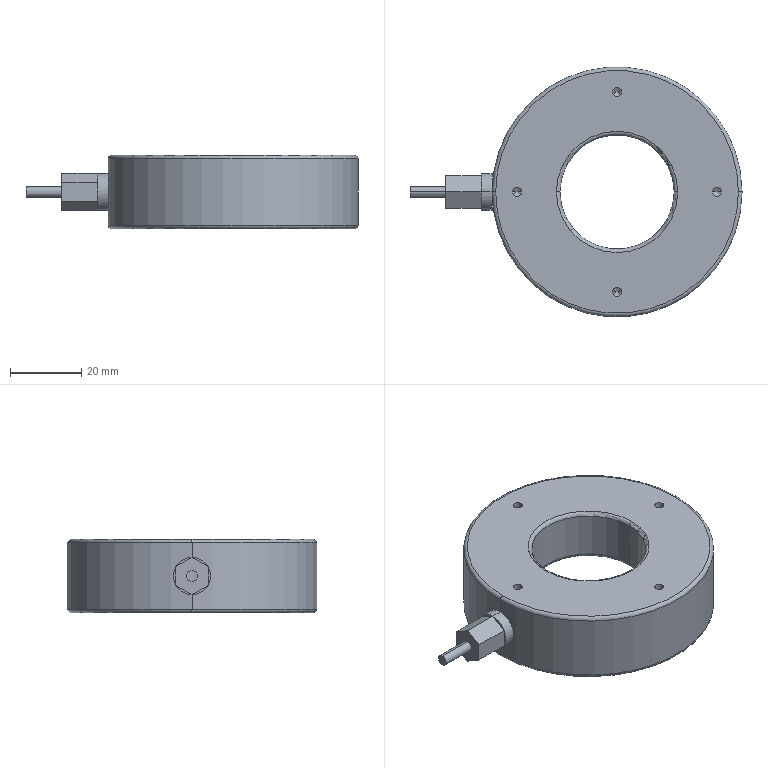Part | STEP file | V-light-HX-A15-D70R3-B-24V | 2 solids | 53 faces | box 93 x 70 x 20.5 mm | volume 59555 mm3 | plane 17 | cylinder 16 | torus 10 | cone 10 | commonest cylinder face diameters 2.5 x8 3 x2 10.4 x2 32 x2 70 x2
STEP:
#1=CARTESIAN_POINT('',(-35.,0.,19.5));
#2=VERTEX_POINT('',#1);
#3=CARTESIAN_POINT('',(35.,0.,19.5));
#4=VERTEX_POINT('',#3);
#5=CARTESIAN_POINT('',(0.,0.,19.5));
#6=DIRECTION('',(0.,0.,-1.));
#7=DIRECTION('',(1.,0.,0.));
#8=AXIS2_PLACEMENT_3D('',#5,#6,#7);
#9=CIRCLE('',#8,35.);
#10=EDGE_CURVE('',#2,#4,#9,.T.);
#11=ORIENTED_EDGE('',*,*,#10,.F.);
#12=CARTESIAN_POINT('',(-34.,0.,20.5));
#13=VERTEX_POINT('',#12);
#14=CARTESIAN_POINT('',(-34.,0.,19.5));
#15=DIRECTION('',(0.,1.,0.));
#16=DIRECTION('',(-1.,0.,0.));
#17=AXIS2_PLACEMENT_3D('',#14,#15,#16);
#18=CIRCLE('',#17,1.);
#19=EDGE_CURVE('',#2,#13,#18,.T.);
#20=ORIENTED_EDGE('',*,*,#19,.T.);
#21=CARTESIAN_POINT('',(34.,0.,20.5));
#22=VERTEX_POINT('',#21);
#23=CARTESIAN_POINT('',(0.,0.,20.5));
#24=DIRECTION('',(0.,0.,1.));
#25=DIRECTION('',(1.,0.,0.));
#26=AXIS2_PLACEMENT_3D('',#23,#24,#25);
#27=CIRCLE('',#26,34.);
#28=EDGE_CURVE('',#22,#13,#27,.T.);
#29=ORIENTED_EDGE('',*,*,#28,.F.);
#30=CARTESIAN_POINT('',(34.,0.,19.5));
#31=DIRECTION('',(0.,-1.,0.));
#32=DIRECTION('',(0.,0.,-1.));
#33=AXIS2_PLACEMENT_3D('',#30,#31,#32);
#34=CIRCLE('',#33,1.);
#35=EDGE_CURVE('',#4,#22,#34,.T.);
#36=ORIENTED_EDGE('',*,*,#35,.F.);
#37=EDGE_LOOP('',(#11,#20,#29,#36));
#38=FACE_OUTER_BOUND('',#37,.T.);
#39=CARTESIAN_POINT('',(0.,0.,19.5));
#40=DIRECTION('',(0.,0.,1.));
#41=DIRECTION('',(1.,0.,0.));
#42=AXIS2_PLACEMENT_3D('',#39,#40,#41);
#43=TOROIDAL_SURFACE('',#42,34.,1.);
#44=ADVANCED_FACE('',(#38),#43,.T.);
#45=CARTESIAN_POINT('',(-34.,0.,0.));
#46=VERTEX_POINT('',#45);
#47=CARTESIAN_POINT('',(34.,0.,0.));
#48=VERTEX_POINT('',#47);
#49=CARTESIAN_POINT('',(0.,0.,0.));
#50=DIRECTION('',(0.,0.,-1.));
#51=DIRECTION('',(1.,0.,0.));
#52=AXIS2_PLACEMENT_3D('',#49,#50,#51);
#53=CIRCLE('',#52,34.);
#54=EDGE_CURVE('',#46,#48,#53,.T.);
#55=ORIENTED_EDGE('',*,*,#54,.F.);
#56=CARTESIAN_POINT('',(-35.,0.,1.));
#57=VERTEX_POINT('',#56);
#58=CARTESIAN_POINT('',(-34.,0.,1.));
#59=DIRECTION('',(0.,1.,0.));
#60=DIRECTION('',(-1.,0.,0.));
#61=AXIS2_PLACEMENT_3D('',#58,#59,#60);
#62=CIRCLE('',#61,1.);
#63=EDGE_CURVE('',#46,#57,#62,.T.);
#64=ORIENTED_EDGE('',*,*,#63,.T.);
#65=CARTESIAN_POINT('',(35.,0.,1.));
#66=VERTEX_POINT('',#65);
#67=CARTESIAN_POINT('',(0.,0.,1.));
#68=DIRECTION('',(0.,0.,1.));
#69=DIRECTION('',(1.,0.,0.));
#70=AXIS2_PLACEMENT_3D('',#67,#68,#69);
#71=CIRCLE('',#70,35.);
#72=EDGE_CURVE('',#66,#57,#71,.T.);
#73=ORIENTED_EDGE('',*,*,#72,.F.);
#74=CARTESIAN_POINT('',(34.,0.,1.));
#75=DIRECTION('',(0.,-1.,0.));
#76=DIRECTION('',(0.,0.,-1.));
#77=AXIS2_PLACEMENT_3D('',#74,#75,#76);
#78=CIRCLE('',#77,1.);
#79=EDGE_CURVE('',#48,#66,#78,.T.);
#80=ORIENTED_EDGE('',*,*,#79,.F.);
#81=EDGE_LOOP('',(#55,#64,#73,#80));
#82=FACE_OUTER_BOUND('',#81,.T.);
#83=CARTESIAN_POINT('',(0.,0.,1.));
#84=DIRECTION('',(0.,0.,1.));
#85=DIRECTION('',(1.,0.,0.));
#86=AXIS2_PLACEMENT_3D('',#83,#84,#85);
#87=TOROIDAL_SURFACE('',#86,34.,1.);
#88=ADVANCED_FACE('',(#82),#87,.T.);
#89=CARTESIAN_POINT('',(-16.,0.,6.566));
#90=VERTEX_POINT('',#89);
#91=CARTESIAN_POINT('',(16.,0.,6.566));
#92=VERTEX_POINT('',#91);
#93=CARTESIAN_POINT('',(0.,0.,6.566));
#94=DIRECTION('',(0.,0.,-1.));
#95=DIRECTION('',(1.,0.,0.));
#96=AXIS2_PLACEMENT_3D('',#93,#94,#95);
#97=CIRCLE('',#96,16.);
#98=EDGE_CURVE('',#90,#92,#97,.T.);
#99=ORIENTED_EDGE('',*,*,#98,.F.);
#100=CARTESIAN_POINT('',(-16.486,0.,5.709));
#101=VERTEX_POINT('',#100);
#102=CARTESIAN_POINT('',(-17.,0.,6.566));
#103=DIRECTION('',(0.,1.,0.));
#104=DIRECTION('',(-1.,0.,0.));
#105=AXIS2_PLACEMENT_3D('',#102,#103,#104);
#106=CIRCLE('',#105,1.);
#107=EDGE_CURVE('',#90,#101,#106,.T.);
#108=ORIENTED_EDGE('',*,*,#107,.T.);
#109=CARTESIAN_POINT('',(16.486,0.,5.709));
#110=VERTEX_POINT('',#109);
#111=CARTESIAN_POINT('',(0.,0.,5.709));
#112=DIRECTION('',(0.,0.,1.));
#113=DIRECTION('',(1.,0.,0.));
#114=AXIS2_PLACEMENT_3D('',#111,#112,#113);
#115=CIRCLE('',#114,16.486);
#116=EDGE_CURVE('',#110,#101,#115,.T.);
#117=ORIENTED_EDGE('',*,*,#116,.F.);
#118=CARTESIAN_POINT('',(17.,0.,6.566));
#119=DIRECTION('',(0.,-1.,0.));
#120=DIRECTION('',(0.,0.,-1.));
#121=AXIS2_PLACEMENT_3D('',#118,#119,#120);
#122=CIRCLE('',#121,1.);
#123=EDGE_CURVE('',#92,#110,#122,.T.);
#124=ORIENTED_EDGE('',*,*,#123,.F.);
#125=EDGE_LOOP('',(#99,#108,#117,#124));
#126=FACE_OUTER_BOUND('',#125,.T.);
#127=CARTESIAN_POINT('',(0.,0.,6.566));
#128=DIRECTION('',(0.,0.,1.));
#129=DIRECTION('',(1.,0.,0.));
#130=AXIS2_PLACEMENT_3D('',#127,#128,#129);
#131=TOROIDAL_SURFACE('',#130,17.,1.);
#132=ADVANCED_FACE('',(#126),#131,.T.);
#133=CARTESIAN_POINT('',(-17.,0.,20.5));
#134=VERTEX_POINT('',#133);
#135=CARTESIAN_POINT('',(17.,0.,20.5));
#136=VERTEX_POINT('',#135);
#137=CARTESIAN_POINT('',(0.,0.,20.5));
#138=DIRECTION('',(0.,0.,-1.));
#139=DIRECTION('',(1.,0.,0.));
#140=AXIS2_PLACEMENT_3D('',#137,#138,#139);
#141=CIRCLE('',#140,17.);
#142=EDGE_CURVE('',#134,#136,#141,.T.);
#143=ORIENTED_EDGE('',*,*,#142,.F.);
#144=CARTESIAN_POINT('',(-16.,0.,19.5));
#145=VERTEX_POINT('',#144);
#146=CARTESIAN_POINT('',(-17.,0.,19.5));
#147=DIRECTION('',(0.,1.,0.));
#148=DIRECTION('',(-1.,0.,0.));
#149=AXIS2_PLACEMENT_3D('',#146,#147,#148);
#150=CIRCLE('',#149,1.);
#151=EDGE_CURVE('',#134,#145,#150,.T.);
#152=ORIENTED_EDGE('',*,*,#151,.T.);
#153=CARTESIAN_POINT('',(16.,0.,19.5));
#154=VERTEX_POINT('',#153);
#155=CARTESIAN_POINT('',(0.,0.,19.5));
#156=DIRECTION('',(0.,0.,1.));
#157=DIRECTION('',(1.,0.,0.));
#158=AXIS2_PLACEMENT_3D('',#155,#156,#157);
#159=CIRCLE('',#158,16.);
#160=EDGE_CURVE('',#154,#145,#159,.T.);
#161=ORIENTED_EDGE('',*,*,#160,.F.);
#162=CARTESIAN_POINT('',(17.,0.,19.5));
#163=DIRECTION('',(0.,-1.,0.));
#164=DIRECTION('',(0.,0.,-1.));
#165=AXIS2_PLACEMENT_3D('',#162,#163,#164);
#166=CIRCLE('',#165,1.);
#167=EDGE_CURVE('',#136,#154,#166,.T.);
#168=ORIENTED_EDGE('',*,*,#167,.F.);
#169=EDGE_LOOP('',(#143,#152,#161,#168));
#170=FACE_OUTER_BOUND('',#169,.T.);
#171=CARTESIAN_POINT('',(0.,0.,19.5));
#172=DIRECTION('',(0.,0.,1.));
#173=DIRECTION('',(1.,0.,0.));
#174=AXIS2_PLACEMENT_3D('',#171,#172,#173);
#175=TOROIDAL_SURFACE('',#174,17.,1.);
#176=ADVANCED_FACE('',(#170),#175,.T.);
#177=CARTESIAN_POINT('',(-25.762,0.,0.1425));
#178=VERTEX_POINT('',#177);
#179=CARTESIAN_POINT('',(25.762,0.,0.1425));
#180=VERTEX_POINT('',#179);
#181=CARTESIAN_POINT('',(0.,0.,0.1425));
#182=DIRECTION('',(0.,0.,-1.));
#183=DIRECTION('',(-1.,0.,0.));
#184=AXIS2_PLACEMENT_3D('',#181,#182,#183);
#185=CIRCLE('',#184,25.762);
#186=EDGE_CURVE('',#178,#180,#185,.T.);
#187=ORIENTED_EDGE('',*,*,#186,.F.);
#188=CARTESIAN_POINT('',(-26.277,0.,0.));
#189=VERTEX_POINT('',#188);
#190=CARTESIAN_POINT('',(-26.277,0.,1.));
#191=DIRECTION('',(0.,1.,0.));
#192=DIRECTION('',(-1.,0.,0.));
#193=AXIS2_PLACEMENT_3D('',#190,#191,#192);
#194=CIRCLE('',#193,1.);
#195=EDGE_CURVE('',#178,#189,#194,.T.);
#196=ORIENTED_EDGE('',*,*,#195,.T.);
#197=CARTESIAN_POINT('',(26.277,0.,0.));
#198=VERTEX_POINT('',#197);
#199=CARTESIAN_POINT('',(0.,0.,0.));
#200=DIRECTION('',(0.,0.,1.));
#201=DIRECTION('',(1.,0.,0.));
#202=AXIS2_PLACEMENT_3D('',#199,#200,#201);
#203=CIRCLE('',#202,26.277);
#204=EDGE_CURVE('',#198,#189,#203,.T.);
#205=ORIENTED_EDGE('',*,*,#204,.F.);
#206=CARTESIAN_POINT('',(26.277,0.,1.));
#207=DIRECTION('',(0.,-1.,0.));
#208=DIRECTION('',(0.,0.,-1.));
#209=AXIS2_PLACEMENT_3D('',#206,#207,#208);
#210=CIRCLE('',#209,1.);
#211=EDGE_CURVE('',#180,#198,#210,.T.);
#212=ORIENTED_EDGE('',*,*,#211,.F.);
#213=EDGE_LOOP('',(#187,#196,#205,#212));
#214=FACE_OUTER_BOUND('',#213,.T.);
#215=CARTESIAN_POINT('',(0.,0.,1.));
#216=DIRECTION('',(0.,0.,1.));
#217=DIRECTION('',(1.,0.,0.));
#218=AXIS2_PLACEMENT_3D('',#215,#216,#217);
#219=TOROIDAL_SURFACE('',#218,26.277,1.);
#220=ADVANCED_FACE('',(#214),#219,.T.);
#221=CARTESIAN_POINT('',(0.,0.,5.709));
#222=DIRECTION('',(0.,0.,1.));
#223=DIRECTION('',(1.,0.,0.));
#224=AXIS2_PLACEMENT_3D('',#221,#222,#223);
#225=CIRCLE('',#224,16.486);
#226=EDGE_CURVE('',#101,#110,#225,.T.);
#227=ORIENTED_EDGE('',*,*,#226,.T.);
#228=CARTESIAN_POINT('',(26.,0.,0.));
#229=DIRECTION('',(0.8575,0.,-0.5145));
#230=VECTOR('',#229,1000.);
#231=LINE('',#228,#230);
#232=EDGE_CURVE('',#110,#180,#231,.T.);
#233=ORIENTED_EDGE('',*,*,#232,.T.);
#234=CARTESIAN_POINT('',(0.,0.,0.1425));
#235=DIRECTION('',(0.,0.,-1.));
#236=DIRECTION('',(-1.,0.,0.));
#237=AXIS2_PLACEMENT_3D('',#234,#235,#236);
#238=CIRCLE('',#237,25.762);
#239=EDGE_CURVE('',#180,#178,#238,.T.);
#240=ORIENTED_EDGE('',*,*,#239,.T.);
#241=CARTESIAN_POINT('',(-26.,0.,0.));
#242=DIRECTION('',(-0.8575,0.,-0.5145));
#243=VECTOR('',#242,1000.);
#244=LINE('',#241,#243);
#245=EDGE_CURVE('',#101,#178,#244,.T.);
#246=ORIENTED_EDGE('',*,*,#245,.F.);
#247=EDGE_LOOP('',(#227,#233,#240,#246));
#248=FACE_OUTER_BOUND('',#247,.T.);
#249=CARTESIAN_POINT('',(0.,0.,0.));
#250=DIRECTION('',(0.,0.,-1.));
#251=DIRECTION('',(-1.,0.,0.));
#252=AXIS2_PLACEMENT_3D('',#249,#250,#251);
#253=CONICAL_SURFACE('',#252,26.,1.03);
#254=ADVANCED_FACE('',(#248),#253,.F.);
#255=CARTESIAN_POINT('',(-1.25,28.,15.));
#256=VERTEX_POINT('',#255);
#257=CARTESIAN_POINT('',(1.25,28.,15.));
#258=VERTEX_POINT('',#257);
#259=CARTESIAN_POINT('',(0.,28.,15.));
#260=DIRECTION('',(0.,0.,1.));
#261=DIRECTION('',(1.,0.,0.));
#262=AXIS2_PLACEMENT_3D('',#259,#260,#261);
#263=CIRCLE('',#262,1.25);
#264=EDGE_CURVE('',#256,#258,#263,.T.);
#265=ORIENTED_EDGE('',*,*,#264,.F.);
#266=CARTESIAN_POINT('',(-1.25,28.,20.5));
#267=VERTEX_POINT('',#266);
#268=CARTESIAN_POINT('',(-1.25,28.,20.5));
#269=DIRECTION('',(0.,0.,1.));
#270=VECTOR('',#269,1000.);
#271=LINE('',#268,#270);
#272=EDGE_CURVE('',#256,#267,#271,.T.);
#273=ORIENTED_EDGE('',*,*,#272,.T.);
#274=CARTESIAN_POINT('',(1.25,28.,20.5));
#275=VERTEX_POINT('',#274);
#276=CARTESIAN_POINT('',(0.,28.,20.5));
#277=DIRECTION('',(0.,0.,1.));
#278=DIRECTION('',(1.,0.,0.));
#279=AXIS2_PLACEMENT_3D('',#276,#277,#278);
#280=CIRCLE('',#279,1.25);
#281=EDGE_CURVE('',#267,#275,#280,.T.);
#282=ORIENTED_EDGE('',*,*,#281,.T.);
#283=CARTESIAN_POINT('',(1.25,28.,20.5));
#284=DIRECTION('',(0.,0.,1.));
#285=VECTOR('',#284,1000.);
#286=LINE('',#283,#285);
#287=EDGE_CURVE('',#258,#275,#286,.T.);
#288=ORIENTED_EDGE('',*,*,#287,.F.);
#289=EDGE_LOOP('',(#265,#273,#282,#288));
#290=FACE_OUTER_BOUND('',#289,.T.);
#291=CARTESIAN_POINT('',(0.,28.,20.5));
#292=DIRECTION('',(0.,0.,1.));
#293=DIRECTION('',(1.,0.,0.));
#294=AXIS2_PLACEMENT_3D('',#291,#292,#293);
#295=CYLINDRICAL_SURFACE('',#294,1.25);
#296=ADVANCED_FACE('',(#290),#295,.F.);
#297=CARTESIAN_POINT('',(0.,28.,14.249));
#298=VERTEX_POINT('',#297);
#299=CARTESIAN_POINT('',(1.25,28.,15.));
#300=DIRECTION('',(0.8572,0.,0.515));
#301=VECTOR('',#300,1000.);
#302=LINE('',#299,#301);
#303=EDGE_CURVE('',#298,#258,#302,.T.);
#304=ORIENTED_EDGE('',*,*,#303,.F.);
#305=CARTESIAN_POINT('',(-1.25,28.,15.));
#306=DIRECTION('',(-0.8572,0.,0.515));
#307=VECTOR('',#306,1000.);
#308=LINE('',#305,#307);
#309=EDGE_CURVE('',#298,#256,#308,.T.);
#310=ORIENTED_EDGE('',*,*,#309,.T.);
#311=ORIENTED_EDGE('',*,*,#264,.T.);
#312=EDGE_LOOP('',(#304,#310,#311));
#313=FACE_OUTER_BOUND('',#312,.T.);
#314=CARTESIAN_POINT('',(0.,28.,15.));
#315=DIRECTION('',(0.,0.,1.));
#316=DIRECTION('',(1.,0.,0.));
#317=AXIS2_PLACEMENT_3D('',#314,#315,#316);
#318=CONICAL_SURFACE('',#317,1.25,1.03);
#319=ADVANCED_FACE('',(#313),#318,.F.);
#320=CARTESIAN_POINT('',(26.75,0.,15.));
#321=VERTEX_POINT('',#320);
#322=CARTESIAN_POINT('',(29.25,0.,15.));
#323=VERTEX_POINT('',#322);
#324=CARTESIAN_POINT('',(28.,0.,15.));
#325=DIRECTION('',(0.,0.,1.));
#326=DIRECTION('',(1.,0.,0.));
#327=AXIS2_PLACEMENT_3D('',#324,#325,#326);
#328=CIRCLE('',#327,1.25);
#329=EDGE_CURVE('',#321,#323,#328,.T.);
#330=ORIENTED_EDGE('',*,*,#329,.F.);
#331=CARTESIAN_POINT('',(26.75,0.,20.5));
#332=VERTEX_POINT('',#331);
#333=CARTESIAN_POINT('',(26.75,0.,20.5));
#334=DIRECTION('',(0.,0.,1.));
#335=VECTOR('',#334,1000.);
#336=LINE('',#333,#335);
#337=EDGE_CURVE('',#321,#332,#336,.T.);
#338=ORIENTED_EDGE('',*,*,#337,.T.);
#339=CARTESIAN_POINT('',(29.25,0.,20.5));
#340=VERTEX_POINT('',#339);
#341=CARTESIAN_POINT('',(28.,0.,20.5));
#342=DIRECTION('',(0.,0.,1.));
#343=DIRECTION('',(1.,0.,0.));
#344=AXIS2_PLACEMENT_3D('',#341,#342,#343);
#345=CIRCLE('',#344,1.25);
#346=EDGE_CURVE('',#332,#340,#345,.T.);
#347=ORIENTED_EDGE('',*,*,#346,.T.);
#348=CARTESIAN_POINT('',(29.25,0.,20.5));
#349=DIRECTION('',(0.,0.,1.));
#350=VECTOR('',#349,1000.);
#351=LINE('',#348,#350);
#352=EDGE_CURVE('',#323,#340,#351,.T.);
#353=ORIENTED_EDGE('',*,*,#352,.F.);
#354=EDGE_LOOP('',(#330,#338,#347,#353));
#355=FACE_OUTER_BOUND('',#354,.T.);
#356=CARTESIAN_POINT('',(28.,0.,20.5));
#357=DIRECTION('',(0.,0.,1.));
#358=DIRECTION('',(1.,0.,0.));
#359=AXIS2_PLACEMENT_3D('',#356,#357,#358);
#360=CYLINDRICAL_SURFACE('',#359,1.25);
#361=ADVANCED_FACE('',(#355),#360,.F.);
#362=CARTESIAN_POINT('',(28.,0.,14.249));
#363=VERTEX_POINT('',#362);
#364=CARTESIAN_POINT('',(29.25,0.,15.));
#365=DIRECTION('',(0.8572,0.,0.515));
#366=VECTOR('',#365,1000.);
#367=LINE('',#364,#366);
#368=EDGE_CURVE('',#363,#323,#367,.T.);
#369=ORIENTED_EDGE('',*,*,#368,.F.);
#370=CARTESIAN_POINT('',(26.75,0.,15.));
#371=DIRECTION('',(-0.8572,0.,0.515));
#372=VECTOR('',#371,1000.);
#373=LINE('',#370,#372);
#374=EDGE_CURVE('',#363,#321,#373,.T.);
#375=ORIENTED_EDGE('',*,*,#374,.T.);
#376=ORIENTED_EDGE('',*,*,#329,.T.);
#377=EDGE_LOOP('',(#369,#375,#376));
#378=FACE_OUTER_BOUND('',#377,.T.);
#379=CARTESIAN_POINT('',(28.,0.,15.));
#380=DIRECTION('',(0.,0.,1.));
#381=DIRECTION('',(1.,0.,0.));
#382=AXIS2_PLACEMENT_3D('',#379,#380,#381);
#383=CONICAL_SURFACE('',#382,1.25,1.03);
#384=ADVANCED_FACE('',(#378),#383,.F.);
#385=CARTESIAN_POINT('',(-1.25,-28.,15.));
#386=VERTEX_POINT('',#385);
#387=CARTESIAN_POINT('',(1.25,-28.,15.));
#388=VERTEX_POINT('',#387);
#389=CARTESIAN_POINT('',(0.,-28.,15.));
#390=DIRECTION('',(0.,0.,1.));
#391=DIRECTION('',(1.,0.,0.));
#392=AXIS2_PLACEMENT_3D('',#389,#390,#391);
#393=CIRCLE('',#392,1.25);
#394=EDGE_CURVE('',#386,#388,#393,.T.);
#395=ORIENTED_EDGE('',*,*,#394,.F.);
#396=CARTESIAN_POINT('',(-1.25,-28.,20.5));
#397=VERTEX_POINT('',#396);
#398=CARTESIAN_POINT('',(-1.25,-28.,20.5));
#399=DIRECTION('',(0.,0.,1.));
#400=VECTOR('',#399,1000.);
#401=LINE('',#398,#400);
#402=EDGE_CURVE('',#386,#397,#401,.T.);
#403=ORIENTED_EDGE('',*,*,#402,.T.);
#404=CARTESIAN_POINT('',(1.25,-28.,20.5));
#405=VERTEX_POINT('',#404);
#406=CARTESIAN_POINT('',(0.,-28.,20.5));
#407=DIRECTION('',(0.,0.,1.));
#408=DIRECTION('',(1.,0.,0.));
#409=AXIS2_PLACEMENT_3D('',#406,#407,#408);
#410=CIRCLE('',#409,1.25);
#411=EDGE_CURVE('',#397,#405,#410,.T.);
#412=ORIENTED_EDGE('',*,*,#411,.T.);
#413=CARTESIAN_POINT('',(1.25,-28.,20.5));
#414=DIRECTION('',(0.,0.,1.));
#415=VECTOR('',#414,1000.);
#416=LINE('',#413,#415);
#417=EDGE_CURVE('',#388,#405,#416,.T.);
#418=ORIENTED_EDGE('',*,*,#417,.F.);
#419=EDGE_LOOP('',(#395,#403,#412,#418));
#420=FACE_OUTER_BOUND('',#419,.T.);
#421=CARTESIAN_POINT('',(0.,-28.,20.5));
#422=DIRECTION('',(0.,0.,1.));
#423=DIRECTION('',(1.,0.,0.));
#424=AXIS2_PLACEMENT_3D('',#421,#422,#423);
#425=CYLINDRICAL_SURFACE('',#424,1.25);
#426=ADVANCED_FACE('',(#420),#425,.F.);
#427=CARTESIAN_POINT('',(0.,-28.,14.249));
#428=VERTEX_POINT('',#427);
#429=CARTESIAN_POINT('',(1.25,-28.,15.));
#430=DIRECTION('',(0.8572,0.,0.515));
#431=VECTOR('',#430,1000.);
#432=LINE('',#429,#431);
#433=EDGE_CURVE('',#428,#388,#432,.T.);
#434=ORIENTED_EDGE('',*,*,#433,.F.);
#435=CARTESIAN_POINT('',(-1.25,-28.,15.));
#436=DIRECTION('',(-0.8572,0.,0.515));
#437=VECTOR('',#436,1000.);
#438=LINE('',#435,#437);
#439=EDGE_CURVE('',#428,#386,#438,.T.);
#440=ORIENTED_EDGE('',*,*,#439,.T.);
#441=ORIENTED_EDGE('',*,*,#394,.T.);
#442=EDGE_LOOP('',(#434,#440,#441));
#443=FACE_OUTER_BOUND('',#442,.T.);
#444=CARTESIAN_POINT('',(0.,-28.,15.));
#445=DIRECTION('',(0.,0.,1.));
#446=DIRECTION('',(1.,0.,0.));
#447=AXIS2_PLACEMENT_3D('',#444,#445,#446);
#448=CONICAL_SURFACE('',#447,1.25,1.03);
#449=ADVANCED_FACE('',(#443),#448,.F.);
#450=CARTESIAN_POINT('',(-29.25,0.,15.));
#451=VERTEX_POINT('',#450);
#452=CARTESIAN_POINT('',(-26.75,0.,15.));
#453=VERTEX_POINT('',#452);
#454=CARTESIAN_POINT('',(-28.,0.,15.));
#455=DIRECTION('',(0.,0.,1.));
#456=DIRECTION('',(1.,0.,0.));
#457=AXIS2_PLACEMENT_3D('',#454,#455,#456);
#458=CIRCLE('',#457,1.25);
#459=EDGE_CURVE('',#451,#453,#458,.T.);
#460=ORIENTED_EDGE('',*,*,#459,.F.);
#461=CARTESIAN_POINT('',(-29.25,0.,20.5));
#462=VERTEX_POINT('',#461);
#463=CARTESIAN_POINT('',(-29.25,0.,20.5));
#464=DIRECTION('',(0.,0.,1.));
#465=VECTOR('',#464,1000.);
#466=LINE('',#463,#465);
#467=EDGE_CURVE('',#451,#462,#466,.T.);
#468=ORIENTED_EDGE('',*,*,#467,.T.);
#469=CARTESIAN_POINT('',(-26.75,0.,20.5));
#470=VERTEX_POINT('',#469);
#471=CARTESIAN_POINT('',(-28.,0.,20.5));
#472=DIRECTION('',(0.,0.,1.));
#473=DIRECTION('',(1.,0.,0.));
#474=AXIS2_PLACEMENT_3D('',#471,#472,#473);
#475=CIRCLE('',#474,1.25);
#476=EDGE_CURVE('',#462,#470,#475,.T.);
#477=ORIENTED_EDGE('',*,*,#476,.T.);
#478=CARTESIAN_POINT('',(-26.75,0.,20.5));
#479=DIRECTION('',(0.,0.,1.));
#480=VECTOR('',#479,1000.);
#481=LINE('',#478,#480);
#482=EDGE_CURVE('',#453,#470,#481,.T.);
#483=ORIENTED_EDGE('',*,*,#482,.F.);
#484=EDGE_LOOP('',(#460,#468,#477,#483));
#485=FACE_OUTER_BOUND('',#484,.T.);
#486=CARTESIAN_POINT('',(-28.,0.,20.5));
#487=DIRECTION('',(0.,0.,1.));
#488=DIRECTION('',(1.,0.,0.));
#489=AXIS2_PLACEMENT_3D('',#486,#487,#488);
#490=CYLINDRICAL_SURFACE('',#489,1.25);
#491=ADVANCED_FACE('',(#485),#490,.F.);
#492=CARTESIAN_POINT('',(-28.,0.,14.249));
#493=VERTEX_POINT('',#492);
#494=CARTESIAN_POINT('',(-26.75,0.,15.));
#495=DIRECTION('',(0.8572,0.,0.515));
#496=VECTOR('',#495,1000.);
#497=LINE('',#494,#496);
#498=EDGE_CURVE('',#493,#453,#497,.T.);
#499=ORIENTED_EDGE('',*,*,#498,.F.);
#500=CARTESIAN_POINT('',(-29.25,0.,15.));
#501=DIRECTION('',(-0.8572,0.,0.515));
#502=VECTOR('',#501,1000.);
#503=LINE('',#500,#502);
#504=EDGE_CURVE('',#493,#451,#503,.T.);
#505=ORIENTED_EDGE('',*,*,#504,.T.);
#506=ORIENTED_EDGE('',*,*,#459,.T.);
#507=EDGE_LOOP('',(#499,#505,#506));
#508=FACE_OUTER_BOUND('',#507,.T.);
#509=CARTESIAN_POINT('',(-28.,0.,15.));
#510=DIRECTION('',(0.,0.,1.));
#511=DIRECTION('',(1.,0.,0.));
#512=AXIS2_PLACEMENT_3D('',#509,#510,#511);
#513=CONICAL_SURFACE('',#512,1.25,1.03);
#514=ADVANCED_FACE('',(#508),#513,.F.);
#515=CARTESIAN_POINT('',(0.,0.,19.5));
#516=DIRECTION('',(0.,0.,1.));
#517=DIRECTION('',(1.,0.,0.));
#518=AXIS2_PLACEMENT_3D('',#515,#516,#517);
#519=CIRCLE('',#518,16.);
#520=EDGE_CURVE('',#145,#154,#519,.T.);
#521=ORIENTED_EDGE('',*,*,#520,.T.);
#522=CARTESIAN_POINT('',(16.,0.,20.5));
#523=DIRECTION('',(0.,0.,-1.));
#524=VECTOR('',#523,1000.);
#525=LINE('',#522,#524);
#526=EDGE_CURVE('',#154,#92,#525,.T.);
#527=ORIENTED_EDGE('',*,*,#526,.T.);
#528=CARTESIAN_POINT('',(0.,0.,6.566));
#529=DIRECTION('',(0.,0.,-1.));
#530=DIRECTION('',(1.,0.,0.));
#531=AXIS2_PLACEMENT_3D('',#528,#529,#530);
#532=CIRCLE('',#531,16.);
#533=EDGE_CURVE('',#92,#90,#532,.T.);
#534=ORIENTED_EDGE('',*,*,#533,.T.);
#535=CARTESIAN_POINT('',(-16.,0.,20.5));
#536=DIRECTION('',(0.,0.,-1.));
#537=VECTOR('',#536,1000.);
#538=LINE('',#535,#537);
#539=EDGE_CURVE('',#145,#90,#538,.T.);
#540=ORIENTED_EDGE('',*,*,#539,.F.);
#541=EDGE_LOOP('',(#521,#527,#534,#540));
#542=FACE_OUTER_BOUND('',#541,.T.);
#543=CARTESIAN_POINT('',(0.,0.,20.5));
#544=DIRECTION('',(0.,0.,-1.));
#545=DIRECTION('',(-1.,0.,0.));
#546=AXIS2_PLACEMENT_3D('',#543,#544,#545);
#547=CYLINDRICAL_SURFACE('',#546,16.);
#548=ADVANCED_FACE('',(#542),#547,.F.);
#549=ORIENTED_EDGE('',*,*,#10,.T.);
#550=CARTESIAN_POINT('',(35.,0.,20.5));
#551=DIRECTION('',(0.,0.,-1.));
#552=VECTOR('',#551,1000.);
#553=LINE('',#550,#552);
#554=EDGE_CURVE('',#4,#66,#553,.T.);
#555=ORIENTED_EDGE('',*,*,#554,.T.);
#556=ORIENTED_EDGE('',*,*,#72,.T.);
#557=CARTESIAN_POINT('',(-35.,0.,20.5));
#558=DIRECTION('',(0.,0.,-1.));
#559=VECTOR('',#558,1000.);
#560=LINE('',#557,#559);
#561=EDGE_CURVE('',#2,#57,#560,.T.);
#562=ORIENTED_EDGE('',*,*,#561,.F.);
#563=EDGE_LOOP('',(#549,#555,#556,#562));
#564=FACE_OUTER_BOUND('',#563,.T.);
#565=CARTESIAN_POINT('',(0.,0.,20.5));
#566=DIRECTION('',(0.,0.,-1.));
#567=DIRECTION('',(-1.,0.,0.));
#568=AXIS2_PLACEMENT_3D('',#565,#566,#567);
#569=CYLINDRICAL_SURFACE('',#568,35.);
#570=ADVANCED_FACE('',(#564),#569,.T.);
#571=CARTESIAN_POINT('',(0.,0.,20.5));
#572=DIRECTION('',(0.,0.,-1.));
#573=DIRECTION('',(1.,0.,0.));
#574=AXIS2_PLACEMENT_3D('',#571,#572,#573);
#575=CIRCLE('',#574,17.);
#576=EDGE_CURVE('',#136,#134,#575,.T.);
#577=ORIENTED_EDGE('',*,*,#576,.T.);
#578=ORIENTED_EDGE('',*,*,#142,.T.);
#579=EDGE_LOOP('',(#577,#578));
#580=FACE_BOUND('',#579,.T.);
#581=ORIENTED_EDGE('',*,*,#28,.T.);
#582=CARTESIAN_POINT('',(0.,0.,20.5));
#583=DIRECTION('',(0.,0.,1.));
#584=DIRECTION('',(1.,0.,0.));
#585=AXIS2_PLACEMENT_3D('',#582,#583,#584);
#586=CIRCLE('',#585,34.);
#587=EDGE_CURVE('',#13,#22,#586,.T.);
#588=ORIENTED_EDGE('',*,*,#587,.T.);
#589=EDGE_LOOP('',(#581,#588));
#590=FACE_OUTER_BOUND('',#589,.T.);
#591=CARTESIAN_POINT('',(0.,28.,20.5));
#592=DIRECTION('',(0.,0.,1.));
#593=DIRECTION('',(1.,0.,0.));
#594=AXIS2_PLACEMENT_3D('',#591,#592,#593);
#595=CIRCLE('',#594,1.25);
#596=EDGE_CURVE('',#275,#267,#595,.T.);
#597=ORIENTED_EDGE('',*,*,#596,.F.);
#598=ORIENTED_EDGE('',*,*,#281,.F.);
#599=EDGE_LOOP('',(#597,#598));
#600=FACE_BOUND('',#599,.T.);
#601=CARTESIAN_POINT('',(28.,0.,20.5));
#602=DIRECTION('',(0.,0.,1.));
#603=DIRECTION('',(1.,0.,0.));
#604=AXIS2_PLACEMENT_3D('',#601,#602,#603);
#605=CIRCLE('',#604,1.25);
#606=EDGE_CURVE('',#340,#332,#605,.T.);
#607=ORIENTED_EDGE('',*,*,#606,.F.);
#608=ORIENTED_EDGE('',*,*,#346,.F.);
#609=EDGE_LOOP('',(#607,#608));
#610=FACE_BOUND('',#609,.T.);
#611=CARTESIAN_POINT('',(0.,-28.,20.5));
#612=DIRECTION('',(0.,0.,1.));
#613=DIRECTION('',(1.,0.,0.));
#614=AXIS2_PLACEMENT_3D('',#611,#612,#613);
#615=CIRCLE('',#614,1.25);
#616=EDGE_CURVE('',#405,#397,#615,.T.);
#617=ORIENTED_EDGE('',*,*,#616,.F.);
#618=ORIENTED_EDGE('',*,*,#411,.F.);
#619=EDGE_LOOP('',(#617,#618));
#620=FACE_BOUND('',#619,.T.);
#621=CARTESIAN_POINT('',(-28.,0.,20.5));
#622=DIRECTION('',(0.,0.,1.));
#623=DIRECTION('',(1.,0.,0.));
#624=AXIS2_PLACEMENT_3D('',#621,#622,#623);
#625=CIRCLE('',#624,1.25);
#626=EDGE_CURVE('',#470,#462,#625,.T.);
#627=ORIENTED_EDGE('',*,*,#626,.F.);
#628=ORIENTED_EDGE('',*,*,#476,.F.);
#629=EDGE_LOOP('',(#627,#628));
#630=FACE_BOUND('',#629,.T.);
#631=CARTESIAN_POINT('',(0.,0.,20.5));
#632=DIRECTION('',(0.,0.,1.));
#633=DIRECTION('',(1.,0.,0.));
#634=AXIS2_PLACEMENT_3D('',#631,#632,#633);
#635=PLANE('',#634);
#636=ADVANCED_FACE('',(#580,#590,#600,#610,#620,#630),#635,.T.);
#637=ORIENTED_EDGE('',*,*,#204,.T.);
#638=CARTESIAN_POINT('',(0.,0.,0.));
#639=DIRECTION('',(0.,0.,1.));
#640=DIRECTION('',(1.,0.,0.));
#641=AXIS2_PLACEMENT_3D('',#638,#639,#640);
#642=CIRCLE('',#641,26.277);
#643=EDGE_CURVE('',#189,#198,#642,.T.);
#644=ORIENTED_EDGE('',*,*,#643,.T.);
#645=EDGE_LOOP('',(#637,#644));
#646=FACE_BOUND('',#645,.T.);
#647=CARTESIAN_POINT('',(0.,0.,0.));
#648=DIRECTION('',(0.,0.,-1.));
#649=DIRECTION('',(1.,0.,0.));
#650=AXIS2_PLACEMENT_3D('',#647,#648,#649);
#651=CIRCLE('',#650,34.);
#652=EDGE_CURVE('',#48,#46,#651,.T.);
#653=ORIENTED_EDGE('',*,*,#652,.T.);
#654=ORIENTED_EDGE('',*,*,#54,.T.);
#655=EDGE_LOOP('',(#653,#654));
#656=FACE_OUTER_BOUND('',#655,.T.);
#657=CARTESIAN_POINT('',(0.,0.,0.));
#658=DIRECTION('',(0.,0.,1.));
#659=DIRECTION('',(1.,0.,0.));
#660=AXIS2_PLACEMENT_3D('',#657,#658,#659);
#661=PLANE('',#660);
#662=ADVANCED_FACE('',(#646,#656),#661,.F.);
#663=ORIENTED_EDGE('',*,*,#554,.F.);
#664=CARTESIAN_POINT('',(0.,0.,19.5));
#665=DIRECTION('',(0.,0.,-1.));
#666=DIRECTION('',(1.,0.,0.));
#667=AXIS2_PLACEMENT_3D('',#664,#665,#666);
#668=CIRCLE('',#667,35.);
#669=EDGE_CURVE('',#4,#2,#668,.T.);
#670=ORIENTED_EDGE('',*,*,#669,.T.);
#671=ORIENTED_EDGE('',*,*,#561,.T.);
#672=CARTESIAN_POINT('',(0.,0.,1.));
#673=DIRECTION('',(0.,0.,1.));
#674=DIRECTION('',(1.,0.,0.));
#675=AXIS2_PLACEMENT_3D('',#672,#673,#674);
#676=CIRCLE('',#675,35.);
#677=EDGE_CURVE('',#57,#66,#676,.T.);
#678=ORIENTED_EDGE('',*,*,#677,.T.);
#679=EDGE_LOOP('',(#663,#670,#671,#678));
#680=FACE_OUTER_BOUND('',#679,.T.);
#681=CARTESIAN_POINT('',(0.,0.,20.5));
#682=DIRECTION('',(0.,0.,-1.));
#683=DIRECTION('',(-1.,0.,0.));
#684=AXIS2_PLACEMENT_3D('',#681,#682,#683);
#685=CYLINDRICAL_SURFACE('',#684,35.);
#686=ADVANCED_FACE('',(#680),#685,.T.);
#687=ORIENTED_EDGE('',*,*,#526,.F.);
#688=ORIENTED_EDGE('',*,*,#160,.T.);
#689=ORIENTED_EDGE('',*,*,#539,.T.);
#690=ORIENTED_EDGE('',*,*,#98,.T.);
#691=EDGE_LOOP('',(#687,#688,#689,#690));
#692=FACE_OUTER_BOUND('',#691,.T.);
#693=CARTESIAN_POINT('',(0.,0.,20.5));
#694=DIRECTION('',(0.,0.,-1.));
#695=DIRECTION('',(-1.,0.,0.));
#696=AXIS2_PLACEMENT_3D('',#693,#694,#695);
#697=CYLINDRICAL_SURFACE('',#696,16.);
#698=ADVANCED_FACE('',(#692),#697,.F.);
#699=ORIENTED_EDGE('',*,*,#504,.F.);
#700=ORIENTED_EDGE('',*,*,#498,.T.);
#701=CARTESIAN_POINT('',(-28.,0.,15.));
#702=DIRECTION('',(0.,0.,1.));
#703=DIRECTION('',(1.,0.,0.));
#704=AXIS2_PLACEMENT_3D('',#701,#702,#703);
#705=CIRCLE('',#704,1.25);
#706=EDGE_CURVE('',#453,#451,#705,.T.);
#707=ORIENTED_EDGE('',*,*,#706,.T.);
#708=EDGE_LOOP('',(#699,#700,#707));
#709=FACE_OUTER_BOUND('',#708,.T.);
#710=CARTESIAN_POINT('',(-28.,0.,15.));
#711=DIRECTION('',(0.,0.,1.));
#712=DIRECTION('',(1.,0.,0.));
#713=AXIS2_PLACEMENT_3D('',#710,#711,#712);
#714=CONICAL_SURFACE('',#713,1.25,1.03);
#715=ADVANCED_FACE('',(#709),#714,.F.);
#716=ORIENTED_EDGE('',*,*,#467,.F.);
#717=ORIENTED_EDGE('',*,*,#706,.F.);
#718=ORIENTED_EDGE('',*,*,#482,.T.);
#719=ORIENTED_EDGE('',*,*,#626,.T.);
#720=EDGE_LOOP('',(#716,#717,#718,#719));
#721=FACE_OUTER_BOUND('',#720,.T.);
#722=CARTESIAN_POINT('',(-28.,0.,20.5));
#723=DIRECTION('',(0.,0.,1.));
#724=DIRECTION('',(1.,0.,0.));
#725=AXIS2_PLACEMENT_3D('',#722,#723,#724);
#726=CYLINDRICAL_SURFACE('',#725,1.25);
#727=ADVANCED_FACE('',(#721),#726,.F.);
#728=ORIENTED_EDGE('',*,*,#439,.F.);
#729=ORIENTED_EDGE('',*,*,#433,.T.);
#730=CARTESIAN_POINT('',(0.,-28.,15.));
#731=DIRECTION('',(0.,0.,1.));
#732=DIRECTION('',(1.,0.,0.));
#733=AXIS2_PLACEMENT_3D('',#730,#731,#732);
#734=CIRCLE('',#733,1.25);
#735=EDGE_CURVE('',#388,#386,#734,.T.);
#736=ORIENTED_EDGE('',*,*,#735,.T.);
#737=EDGE_LOOP('',(#728,#729,#736));
#738=FACE_OUTER_BOUND('',#737,.T.);
#739=CARTESIAN_POINT('',(0.,-28.,15.));
#740=DIRECTION('',(0.,0.,1.));
#741=DIRECTION('',(1.,0.,0.));
#742=AXIS2_PLACEMENT_3D('',#739,#740,#741);
#743=CONICAL_SURFACE('',#742,1.25,1.03);
#744=ADVANCED_FACE('',(#738),#743,.F.);
#745=ORIENTED_EDGE('',*,*,#402,.F.);
#746=ORIENTED_EDGE('',*,*,#735,.F.);
#747=ORIENTED_EDGE('',*,*,#417,.T.);
#748=ORIENTED_EDGE('',*,*,#616,.T.);
#749=EDGE_LOOP('',(#745,#746,#747,#748));
#750=FACE_OUTER_BOUND('',#749,.T.);
#751=CARTESIAN_POINT('',(0.,-28.,20.5));
#752=DIRECTION('',(0.,0.,1.));
#753=DIRECTION('',(1.,0.,0.));
#754=AXIS2_PLACEMENT_3D('',#751,#752,#753);
#755=CYLINDRICAL_SURFACE('',#754,1.25);
#756=ADVANCED_FACE('',(#750),#755,.F.);
#757=ORIENTED_EDGE('',*,*,#374,.F.);
#758=ORIENTED_EDGE('',*,*,#368,.T.);
#759=CARTESIAN_POINT('',(28.,0.,15.));
#760=DIRECTION('',(0.,0.,1.));
#761=DIRECTION('',(1.,0.,0.));
#762=AXIS2_PLACEMENT_3D('',#759,#760,#761);
#763=CIRCLE('',#762,1.25);
#764=EDGE_CURVE('',#323,#321,#763,.T.);
#765=ORIENTED_EDGE('',*,*,#764,.T.);
#766=EDGE_LOOP('',(#757,#758,#765));
#767=FACE_OUTER_BOUND('',#766,.T.);
#768=CARTESIAN_POINT('',(28.,0.,15.));
#769=DIRECTION('',(0.,0.,1.));
#770=DIRECTION('',(1.,0.,0.));
#771=AXIS2_PLACEMENT_3D('',#768,#769,#770);
#772=CONICAL_SURFACE('',#771,1.25,1.03);
#773=ADVANCED_FACE('',(#767),#772,.F.);
#774=ORIENTED_EDGE('',*,*,#337,.F.);
#775=ORIENTED_EDGE('',*,*,#764,.F.);
#776=ORIENTED_EDGE('',*,*,#352,.T.);
#777=ORIENTED_EDGE('',*,*,#606,.T.);
#778=EDGE_LOOP('',(#774,#775,#776,#777));
#779=FACE_OUTER_BOUND('',#778,.T.);
#780=CARTESIAN_POINT('',(28.,0.,20.5));
#781=DIRECTION('',(0.,0.,1.));
#782=DIRECTION('',(1.,0.,0.));
#783=AXIS2_PLACEMENT_3D('',#780,#781,#782);
#784=CYLINDRICAL_SURFACE('',#783,1.25);
#785=ADVANCED_FACE('',(#779),#784,.F.);
#786=ORIENTED_EDGE('',*,*,#309,.F.);
#787=ORIENTED_EDGE('',*,*,#303,.T.);
#788=CARTESIAN_POINT('',(0.,28.,15.));
#789=DIRECTION('',(0.,0.,1.));
#790=DIRECTION('',(1.,0.,0.));
#791=AXIS2_PLACEMENT_3D('',#788,#789,#790);
#792=CIRCLE('',#791,1.25);
#793=EDGE_CURVE('',#258,#256,#792,.T.);
#794=ORIENTED_EDGE('',*,*,#793,.T.);
#795=EDGE_LOOP('',(#786,#787,#794));
#796=FACE_OUTER_BOUND('',#795,.T.);
#797=CARTESIAN_POINT('',(0.,28.,15.));
#798=DIRECTION('',(0.,0.,1.));
#799=DIRECTION('',(1.,0.,0.));
#800=AXIS2_PLACEMENT_3D('',#797,#798,#799);
#801=CONICAL_SURFACE('',#800,1.25,1.03);
#802=ADVANCED_FACE('',(#796),#801,.F.);
#803=ORIENTED_EDGE('',*,*,#272,.F.);
#804=ORIENTED_EDGE('',*,*,#793,.F.);
#805=ORIENTED_EDGE('',*,*,#287,.T.);
#806=ORIENTED_EDGE('',*,*,#596,.T.);
#807=EDGE_LOOP('',(#803,#804,#805,#806));
#808=FACE_OUTER_BOUND('',#807,.T.);
#809=CARTESIAN_POINT('',(0.,28.,20.5));
#810=DIRECTION('',(0.,0.,1.));
#811=DIRECTION('',(1.,0.,0.));
#812=AXIS2_PLACEMENT_3D('',#809,#810,#811);
#813=CYLINDRICAL_SURFACE('',#812,1.25);
#814=ADVANCED_FACE('',(#808),#813,.F.);
#815=ORIENTED_EDGE('',*,*,#232,.F.);
#816=ORIENTED_EDGE('',*,*,#116,.T.);
#817=ORIENTED_EDGE('',*,*,#245,.T.);
#818=ORIENTED_EDGE('',*,*,#186,.T.);
#819=EDGE_LOOP('',(#815,#816,#817,#818));
#820=FACE_OUTER_BOUND('',#819,.T.);
#821=CARTESIAN_POINT('',(0.,0.,0.));
#822=DIRECTION('',(0.,0.,-1.));
#823=DIRECTION('',(-1.,0.,0.));
#824=AXIS2_PLACEMENT_3D('',#821,#822,#823);
#825=CONICAL_SURFACE('',#824,26.,1.03);
#826=ADVANCED_FACE('',(#820),#825,.F.);
#827=ORIENTED_EDGE('',*,*,#195,.F.);
#828=ORIENTED_EDGE('',*,*,#239,.F.);
#829=ORIENTED_EDGE('',*,*,#211,.T.);
#830=ORIENTED_EDGE('',*,*,#643,.F.);
#831=EDGE_LOOP('',(#827,#828,#829,#830));
#832=FACE_OUTER_BOUND('',#831,.T.);
#833=CARTESIAN_POINT('',(0.,0.,1.));
#834=DIRECTION('',(0.,0.,1.));
#835=DIRECTION('',(1.,0.,0.));
#836=AXIS2_PLACEMENT_3D('',#833,#834,#835);
#837=TOROIDAL_SURFACE('',#836,26.277,1.);
#838=ADVANCED_FACE('',(#832),#837,.T.);
#839=ORIENTED_EDGE('',*,*,#151,.F.);
#840=ORIENTED_EDGE('',*,*,#576,.F.);
#841=ORIENTED_EDGE('',*,*,#167,.T.);
#842=ORIENTED_EDGE('',*,*,#520,.F.);
#843=EDGE_LOOP('',(#839,#840,#841,#842));
#844=FACE_OUTER_BOUND('',#843,.T.);
#845=CARTESIAN_POINT('',(0.,0.,19.5));
#846=DIRECTION('',(0.,0.,1.));
#847=DIRECTION('',(1.,0.,0.));
#848=AXIS2_PLACEMENT_3D('',#845,#846,#847);
#849=TOROIDAL_SURFACE('',#848,17.,1.);
#850=ADVANCED_FACE('',(#844),#849,.T.);
#851=ORIENTED_EDGE('',*,*,#107,.F.);
#852=ORIENTED_EDGE('',*,*,#533,.F.);
#853=ORIENTED_EDGE('',*,*,#123,.T.);
#854=ORIENTED_EDGE('',*,*,#226,.F.);
#855=EDGE_LOOP('',(#851,#852,#853,#854));
#856=FACE_OUTER_BOUND('',#855,.T.);
#857=CARTESIAN_POINT('',(0.,0.,6.566));
#858=DIRECTION('',(0.,0.,1.));
#859=DIRECTION('',(1.,0.,0.));
#860=AXIS2_PLACEMENT_3D('',#857,#858,#859);
#861=TOROIDAL_SURFACE('',#860,17.,1.);
#862=ADVANCED_FACE('',(#856),#861,.T.);
#863=ORIENTED_EDGE('',*,*,#63,.F.);
#864=ORIENTED_EDGE('',*,*,#652,.F.);
#865=ORIENTED_EDGE('',*,*,#79,.T.);
#866=ORIENTED_EDGE('',*,*,#677,.F.);
#867=EDGE_LOOP('',(#863,#864,#865,#866));
#868=FACE_OUTER_BOUND('',#867,.T.);
#869=CARTESIAN_POINT('',(0.,0.,1.));
#870=DIRECTION('',(0.,0.,1.));
#871=DIRECTION('',(1.,0.,0.));
#872=AXIS2_PLACEMENT_3D('',#869,#870,#871);
#873=TOROIDAL_SURFACE('',#872,34.,1.);
#874=ADVANCED_FACE('',(#868),#873,.T.);
#875=ORIENTED_EDGE('',*,*,#19,.F.);
#876=ORIENTED_EDGE('',*,*,#669,.F.);
#877=ORIENTED_EDGE('',*,*,#35,.T.);
#878=ORIENTED_EDGE('',*,*,#587,.F.);
#879=EDGE_LOOP('',(#875,#876,#877,#878));
#880=FACE_OUTER_BOUND('',#879,.T.);
#881=CARTESIAN_POINT('',(0.,0.,19.5));
#882=DIRECTION('',(0.,0.,1.));
#883=DIRECTION('',(1.,0.,0.));
#884=AXIS2_PLACEMENT_3D('',#881,#882,#883);
#885=TOROIDAL_SURFACE('',#884,34.,1.);
#886=ADVANCED_FACE('',(#880),#885,.T.);
#887=CLOSED_SHELL('',(#44,#88,#132,#176,#220,#254,#296,#319,#361,#384,#426,#449,#491,#514,#548,#570,#636,#662,#686,#698,#715,#727,#744,#756,#773,#785,#802,#814,#826,#838,#850,#862,#874,#886));
#888=MANIFOLD_SOLID_BREP('',#887);
#889=CARTESIAN_POINT('',(-58.,0.,11.75));
#890=VERTEX_POINT('',#889);
#891=CARTESIAN_POINT('',(-58.,0.,8.75));
#892=VERTEX_POINT('',#891);
#893=CARTESIAN_POINT('',(-58.,0.,10.25));
#894=DIRECTION('',(-1.,0.,0.));
#895=DIRECTION('',(0.,0.,1.));
#896=AXIS2_PLACEMENT_3D('',#893,#894,#895);
#897=CIRCLE('',#896,1.5);
#898=EDGE_CURVE('',#890,#892,#897,.T.);
#899=ORIENTED_EDGE('',*,*,#898,.F.);
#900=CARTESIAN_POINT('',(-48.,0.,11.75));
#901=VERTEX_POINT('',#900);
#902=CARTESIAN_POINT('',(-58.,0.,11.75));
#903=DIRECTION('',(1.,0.,0.));
#904=VECTOR('',#903,1000.);
#905=LINE('',#902,#904);
#906=EDGE_CURVE('',#890,#901,#905,.T.);
#907=ORIENTED_EDGE('',*,*,#906,.T.);
#908=CARTESIAN_POINT('',(-48.,0.,8.75));
#909=VERTEX_POINT('',#908);
#910=CARTESIAN_POINT('',(-48.,0.,10.25));
#911=DIRECTION('',(-1.,0.,0.));
#912=DIRECTION('',(0.,0.,1.));
#913=AXIS2_PLACEMENT_3D('',#910,#911,#912);
#914=CIRCLE('',#913,1.5);
#915=EDGE_CURVE('',#901,#909,#914,.T.);
#916=ORIENTED_EDGE('',*,*,#915,.T.);
#917=CARTESIAN_POINT('',(-58.,0.,8.75));
#918=DIRECTION('',(1.,0.,0.));
#919=VECTOR('',#918,1000.);
#920=LINE('',#917,#919);
#921=EDGE_CURVE('',#892,#909,#920,.T.);
#922=ORIENTED_EDGE('',*,*,#921,.F.);
#923=EDGE_LOOP('',(#899,#907,#916,#922));
#924=FACE_OUTER_BOUND('',#923,.T.);
#925=CARTESIAN_POINT('',(-58.,0.,10.25));
#926=DIRECTION('',(1.,0.,0.));
#927=DIRECTION('',(0.,0.,-1.));
#928=AXIS2_PLACEMENT_3D('',#925,#926,#927);
#929=CYLINDRICAL_SURFACE('',#928,1.5);
#930=ADVANCED_FACE('',(#924),#929,.T.);
#931=CARTESIAN_POINT('',(-38.,0.,15.45));
#932=VERTEX_POINT('',#931);
#933=CARTESIAN_POINT('',(-38.,4.503,12.85));
#934=VERTEX_POINT('',#933);
#935=CARTESIAN_POINT('',(-38.,0.,10.25));
#936=DIRECTION('',(-1.,0.,0.));
#937=DIRECTION('',(0.,0.,1.));
#938=AXIS2_PLACEMENT_3D('',#935,#936,#937);
#939=CIRCLE('',#938,5.2);
#940=EDGE_CURVE('',#932,#934,#939,.T.);
#941=ORIENTED_EDGE('',*,*,#940,.F.);
#942=CARTESIAN_POINT('',(-35.,0.,15.45));
#943=VERTEX_POINT('',#942);
#944=CARTESIAN_POINT('',(-48.,0.,15.45));
#945=DIRECTION('',(1.,0.,0.));
#946=VECTOR('',#945,1000.);
#947=LINE('',#944,#946);
#948=EDGE_CURVE('',#932,#943,#947,.T.);
#949=ORIENTED_EDGE('',*,*,#948,.T.);
#950=CARTESIAN_POINT('',(-35.,0.,5.05));
#951=VERTEX_POINT('',#950);
#952=CARTESIAN_POINT('',(-35.,0.,10.25));
#953=DIRECTION('',(-1.,0.,0.));
#954=DIRECTION('',(0.,0.,1.));
#955=AXIS2_PLACEMENT_3D('',#952,#953,#954);
#956=CIRCLE('',#955,5.2);
#957=EDGE_CURVE('',#943,#951,#956,.T.);
#958=ORIENTED_EDGE('',*,*,#957,.T.);
#959=CARTESIAN_POINT('',(-38.,0.,5.05));
#960=VERTEX_POINT('',#959);
#961=CARTESIAN_POINT('',(-48.,0.,5.05));
#962=DIRECTION('',(1.,0.,0.));
#963=VECTOR('',#962,1000.);
#964=LINE('',#961,#963);
#965=EDGE_CURVE('',#960,#951,#964,.T.);
#966=ORIENTED_EDGE('',*,*,#965,.F.);
#967=CARTESIAN_POINT('',(-38.,4.503,7.65));
#968=VERTEX_POINT('',#967);
#969=CARTESIAN_POINT('',(-38.,0.,10.25));
#970=DIRECTION('',(-1.,0.,0.));
#971=DIRECTION('',(0.,0.,1.));
#972=AXIS2_PLACEMENT_3D('',#969,#970,#971);
#973=CIRCLE('',#972,5.2);
#974=EDGE_CURVE('',#968,#960,#973,.T.);
#975=ORIENTED_EDGE('',*,*,#974,.F.);
#976=CARTESIAN_POINT('',(-38.,0.,10.25));
#977=DIRECTION('',(-1.,0.,0.));
#978=DIRECTION('',(0.,0.,1.));
#979=AXIS2_PLACEMENT_3D('',#976,#977,#978);
#980=CIRCLE('',#979,5.2);
#981=EDGE_CURVE('',#934,#968,#980,.T.);
#982=ORIENTED_EDGE('',*,*,#981,.F.);
#983=EDGE_LOOP('',(#941,#949,#958,#966,#975,#982));
#984=FACE_OUTER_BOUND('',#983,.T.);
#985=CARTESIAN_POINT('',(-48.,0.,10.25));
#986=DIRECTION('',(1.,0.,0.));
#987=DIRECTION('',(0.,0.,-1.));
#988=AXIS2_PLACEMENT_3D('',#985,#986,#987);
#989=CYLINDRICAL_SURFACE('',#988,5.2);
#990=ADVANCED_FACE('',(#984),#989,.T.);
#991=CARTESIAN_POINT('',(-48.,-4.503,7.65));
#992=VERTEX_POINT('',#991);
#993=CARTESIAN_POINT('',(-48.,-4.503,12.85));
#994=VERTEX_POINT('',#993);
#995=CARTESIAN_POINT('',(-48.,-4.503,7.65));
#996=DIRECTION('',(0.,0.,1.));
#997=VECTOR('',#996,1000.);
#998=LINE('',#995,#997);
#999=EDGE_CURVE('',#992,#994,#998,.T.);
#1000=ORIENTED_EDGE('',*,*,#999,.T.);
#1001=CARTESIAN_POINT('',(-48.,0.,15.45));
#1002=VERTEX_POINT('',#1001);
#1003=CARTESIAN_POINT('',(-48.,-4.503,12.85));
#1004=DIRECTION('',(0.,0.866,0.5));
#1005=VECTOR('',#1004,1000.);
#1006=LINE('',#1003,#1005);
#1007=EDGE_CURVE('',#994,#1002,#1006,.T.);
#1008=ORIENTED_EDGE('',*,*,#1007,.T.);
#1009=CARTESIAN_POINT('',(-48.,4.503,12.85));
#1010=VERTEX_POINT('',#1009);
#1011=CARTESIAN_POINT('',(-48.,0.,15.45));
#1012=DIRECTION('',(0.,0.866,-0.5));
#1013=VECTOR('',#1012,1000.);
#1014=LINE('',#1011,#1013);
#1015=EDGE_CURVE('',#1002,#1010,#1014,.T.);
#1016=ORIENTED_EDGE('',*,*,#1015,.T.);
#1017=CARTESIAN_POINT('',(-48.,4.503,7.65));
#1018=VERTEX_POINT('',#1017);
#1019=CARTESIAN_POINT('',(-48.,4.503,12.85));
#1020=DIRECTION('',(0.,0.,-1.));
#1021=VECTOR('',#1020,1000.);
#1022=LINE('',#1019,#1021);
#1023=EDGE_CURVE('',#1010,#1018,#1022,.T.);
#1024=ORIENTED_EDGE('',*,*,#1023,.T.);
#1025=CARTESIAN_POINT('',(-48.,0.,5.05));
#1026=VERTEX_POINT('',#1025);
#1027=CARTESIAN_POINT('',(-48.,4.503,7.65));
#1028=DIRECTION('',(0.,-0.866,-0.5));
#1029=VECTOR('',#1028,1000.);
#1030=LINE('',#1027,#1029);
#1031=EDGE_CURVE('',#1018,#1026,#1030,.T.);
#1032=ORIENTED_EDGE('',*,*,#1031,.T.);
#1033=CARTESIAN_POINT('',(-48.,0.,5.05));
#1034=DIRECTION('',(0.,-0.866,0.5));
#1035=VECTOR('',#1034,1000.);
#1036=LINE('',#1033,#1035);
#1037=EDGE_CURVE('',#1026,#992,#1036,.T.);
#1038=ORIENTED_EDGE('',*,*,#1037,.T.);
#1039=EDGE_LOOP('',(#1000,#1008,#1016,#1024,#1032,#1038));
#1040=FACE_OUTER_BOUND('',#1039,.T.);
#1041=CARTESIAN_POINT('',(-48.,0.,10.25));
#1042=DIRECTION('',(-1.,0.,0.));
#1043=DIRECTION('',(0.,0.,1.));
#1044=AXIS2_PLACEMENT_3D('',#1041,#1042,#1043);
#1045=CIRCLE('',#1044,1.5);
#1046=EDGE_CURVE('',#909,#901,#1045,.T.);
#1047=ORIENTED_EDGE('',*,*,#1046,.F.);
#1048=ORIENTED_EDGE('',*,*,#915,.F.);
#1049=EDGE_LOOP('',(#1047,#1048));
#1050=FACE_BOUND('',#1049,.T.);
#1051=CARTESIAN_POINT('',(-48.,0.,10.25));
#1052=DIRECTION('',(-1.,0.,0.));
#1053=DIRECTION('',(0.,0.,1.));
#1054=AXIS2_PLACEMENT_3D('',#1051,#1052,#1053);
#1055=PLANE('',#1054);
#1056=ADVANCED_FACE('',(#1040,#1050),#1055,.T.);
#1057=ORIENTED_EDGE('',*,*,#948,.F.);
#1058=CARTESIAN_POINT('',(-38.,-4.503,12.85));
#1059=VERTEX_POINT('',#1058);
#1060=CARTESIAN_POINT('',(-38.,0.,10.25));
#1061=DIRECTION('',(-1.,0.,0.));
#1062=DIRECTION('',(0.,0.,1.));
#1063=AXIS2_PLACEMENT_3D('',#1060,#1061,#1062);
#1064=CIRCLE('',#1063,5.2);
#1065=EDGE_CURVE('',#1059,#932,#1064,.T.);
#1066=ORIENTED_EDGE('',*,*,#1065,.F.);
#1067=CARTESIAN_POINT('',(-38.,-4.503,7.65));
#1068=VERTEX_POINT('',#1067);
#1069=CARTESIAN_POINT('',(-38.,0.,10.25));
#1070=DIRECTION('',(-1.,0.,0.));
#1071=DIRECTION('',(0.,0.,1.));
#1072=AXIS2_PLACEMENT_3D('',#1069,#1070,#1071);
#1073=CIRCLE('',#1072,5.2);
#1074=EDGE_CURVE('',#1068,#1059,#1073,.T.);
#1075=ORIENTED_EDGE('',*,*,#1074,.F.);
#1076=CARTESIAN_POINT('',(-38.,0.,10.25));
#1077=DIRECTION('',(-1.,0.,0.));
#1078=DIRECTION('',(0.,0.,1.));
#1079=AXIS2_PLACEMENT_3D('',#1076,#1077,#1078);
#1080=CIRCLE('',#1079,5.2);
#1081=EDGE_CURVE('',#960,#1068,#1080,.T.);
#1082=ORIENTED_EDGE('',*,*,#1081,.F.);
#1083=ORIENTED_EDGE('',*,*,#965,.T.);
#1084=CARTESIAN_POINT('',(-35.,0.,10.25));
#1085=DIRECTION('',(-1.,0.,0.));
#1086=DIRECTION('',(0.,0.,1.));
#1087=AXIS2_PLACEMENT_3D('',#1084,#1085,#1086);
#1088=CIRCLE('',#1087,5.2);
#1089=EDGE_CURVE('',#951,#943,#1088,.T.);
#1090=ORIENTED_EDGE('',*,*,#1089,.T.);
#1091=EDGE_LOOP('',(#1057,#1066,#1075,#1082,#1083,#1090));
#1092=FACE_OUTER_BOUND('',#1091,.T.);
#1093=CARTESIAN_POINT('',(-48.,0.,10.25));
#1094=DIRECTION('',(1.,0.,0.));
#1095=DIRECTION('',(0.,0.,-1.));
#1096=AXIS2_PLACEMENT_3D('',#1093,#1094,#1095);
#1097=CYLINDRICAL_SURFACE('',#1096,5.2);
#1098=ADVANCED_FACE('',(#1092),#1097,.T.);
#1099=ORIENTED_EDGE('',*,*,#1089,.F.);
#1100=ORIENTED_EDGE('',*,*,#957,.F.);
#1101=EDGE_LOOP('',(#1099,#1100));
#1102=FACE_OUTER_BOUND('',#1101,.T.);
#1103=CARTESIAN_POINT('',(-35.,0.,10.25));
#1104=DIRECTION('',(-1.,0.,0.));
#1105=DIRECTION('',(0.,0.,1.));
#1106=AXIS2_PLACEMENT_3D('',#1103,#1104,#1105);
#1107=PLANE('',#1106);
#1108=ADVANCED_FACE('',(#1102),#1107,.F.);
#1109=ORIENTED_EDGE('',*,*,#940,.T.);
#1110=CARTESIAN_POINT('',(-38.,0.,15.45));
#1111=DIRECTION('',(0.,0.866,-0.5));
#1112=VECTOR('',#1111,1000.);
#1113=LINE('',#1110,#1112);
#1114=EDGE_CURVE('',#932,#934,#1113,.T.);
#1115=ORIENTED_EDGE('',*,*,#1114,.F.);
#1116=EDGE_LOOP('',(#1109,#1115));
#1117=FACE_OUTER_BOUND('',#1116,.T.);
#1118=CARTESIAN_POINT('',(-38.,0.,10.25));
#1119=DIRECTION('',(-1.,0.,0.));
#1120=DIRECTION('',(0.,0.,1.));
#1121=AXIS2_PLACEMENT_3D('',#1118,#1119,#1120);
#1122=PLANE('',#1121);
#1123=ADVANCED_FACE('',(#1117),#1122,.T.);
#1124=ORIENTED_EDGE('',*,*,#981,.T.);
#1125=CARTESIAN_POINT('',(-38.,4.503,12.85));
#1126=DIRECTION('',(0.,0.,-1.));
#1127=VECTOR('',#1126,1000.);
#1128=LINE('',#1125,#1127);
#1129=EDGE_CURVE('',#934,#968,#1128,.T.);
#1130=ORIENTED_EDGE('',*,*,#1129,.F.);
#1131=EDGE_LOOP('',(#1124,#1130));
#1132=FACE_OUTER_BOUND('',#1131,.T.);
#1133=CARTESIAN_POINT('',(-38.,0.,10.25));
#1134=DIRECTION('',(-1.,0.,0.));
#1135=DIRECTION('',(0.,0.,1.));
#1136=AXIS2_PLACEMENT_3D('',#1133,#1134,#1135);
#1137=PLANE('',#1136);
#1138=ADVANCED_FACE('',(#1132),#1137,.T.);
#1139=ORIENTED_EDGE('',*,*,#974,.T.);
#1140=CARTESIAN_POINT('',(-38.,4.503,7.65));
#1141=DIRECTION('',(0.,-0.866,-0.5));
#1142=VECTOR('',#1141,1000.);
#1143=LINE('',#1140,#1142);
#1144=EDGE_CURVE('',#968,#960,#1143,.T.);
#1145=ORIENTED_EDGE('',*,*,#1144,.F.);
#1146=EDGE_LOOP('',(#1139,#1145));
#1147=FACE_OUTER_BOUND('',#1146,.T.);
#1148=CARTESIAN_POINT('',(-38.,0.,10.25));
#1149=DIRECTION('',(-1.,0.,0.));
#1150=DIRECTION('',(0.,0.,1.));
#1151=AXIS2_PLACEMENT_3D('',#1148,#1149,#1150);
#1152=PLANE('',#1151);
#1153=ADVANCED_FACE('',(#1147),#1152,.T.);
#1154=ORIENTED_EDGE('',*,*,#1081,.T.);
#1155=CARTESIAN_POINT('',(-38.,0.,5.05));
#1156=DIRECTION('',(0.,-0.866,0.5));
#1157=VECTOR('',#1156,1000.);
#1158=LINE('',#1155,#1157);
#1159=EDGE_CURVE('',#960,#1068,#1158,.T.);
#1160=ORIENTED_EDGE('',*,*,#1159,.F.);
#1161=EDGE_LOOP('',(#1154,#1160));
#1162=FACE_OUTER_BOUND('',#1161,.T.);
#1163=CARTESIAN_POINT('',(-38.,0.,10.25));
#1164=DIRECTION('',(-1.,0.,0.));
#1165=DIRECTION('',(0.,0.,1.));
#1166=AXIS2_PLACEMENT_3D('',#1163,#1164,#1165);
#1167=PLANE('',#1166);
#1168=ADVANCED_FACE('',(#1162),#1167,.T.);
#1169=ORIENTED_EDGE('',*,*,#1074,.T.);
#1170=CARTESIAN_POINT('',(-38.,-4.503,7.65));
#1171=DIRECTION('',(0.,0.,1.));
#1172=VECTOR('',#1171,1000.);
#1173=LINE('',#1170,#1172);
#1174=EDGE_CURVE('',#1068,#1059,#1173,.T.);
#1175=ORIENTED_EDGE('',*,*,#1174,.F.);
#1176=EDGE_LOOP('',(#1169,#1175));
#1177=FACE_OUTER_BOUND('',#1176,.T.);
#1178=CARTESIAN_POINT('',(-38.,0.,10.25));
#1179=DIRECTION('',(-1.,0.,0.));
#1180=DIRECTION('',(0.,0.,1.));
#1181=AXIS2_PLACEMENT_3D('',#1178,#1179,#1180);
#1182=PLANE('',#1181);
#1183=ADVANCED_FACE('',(#1177),#1182,.T.);
#1184=ORIENTED_EDGE('',*,*,#1065,.T.);
#1185=CARTESIAN_POINT('',(-38.,-4.503,12.85));
#1186=DIRECTION('',(0.,0.866,0.5));
#1187=VECTOR('',#1186,1000.);
#1188=LINE('',#1185,#1187);
#1189=EDGE_CURVE('',#1059,#932,#1188,.T.);
#1190=ORIENTED_EDGE('',*,*,#1189,.F.);
#1191=EDGE_LOOP('',(#1184,#1190));
#1192=FACE_OUTER_BOUND('',#1191,.T.);
#1193=CARTESIAN_POINT('',(-38.,0.,10.25));
#1194=DIRECTION('',(-1.,0.,0.));
#1195=DIRECTION('',(0.,0.,1.));
#1196=AXIS2_PLACEMENT_3D('',#1193,#1194,#1195);
#1197=PLANE('',#1196);
#1198=ADVANCED_FACE('',(#1192),#1197,.T.);
#1199=ORIENTED_EDGE('',*,*,#1007,.F.);
#1200=CARTESIAN_POINT('',(-38.,-4.503,12.85));
#1201=DIRECTION('',(-1.,0.,0.));
#1202=VECTOR('',#1201,1000.);
#1203=LINE('',#1200,#1202);
#1204=EDGE_CURVE('',#1059,#994,#1203,.T.);
#1205=ORIENTED_EDGE('',*,*,#1204,.F.);
#1206=ORIENTED_EDGE('',*,*,#1189,.T.);
#1207=CARTESIAN_POINT('',(-38.,0.,15.45));
#1208=DIRECTION('',(-1.,0.,0.));
#1209=VECTOR('',#1208,1000.);
#1210=LINE('',#1207,#1209);
#1211=EDGE_CURVE('',#932,#1002,#1210,.T.);
#1212=ORIENTED_EDGE('',*,*,#1211,.T.);
#1213=EDGE_LOOP('',(#1199,#1205,#1206,#1212));
#1214=FACE_OUTER_BOUND('',#1213,.T.);
#1215=CARTESIAN_POINT('',(-38.,-4.503,12.85));
#1216=DIRECTION('',(0.,-0.5,0.866));
#1217=DIRECTION('',(0.,-0.866,-0.5));
#1218=AXIS2_PLACEMENT_3D('',#1215,#1216,#1217);
#1219=PLANE('',#1218);
#1220=ADVANCED_FACE('',(#1214),#1219,.T.);
#1221=ORIENTED_EDGE('',*,*,#999,.F.);
#1222=CARTESIAN_POINT('',(-38.,-4.503,7.65));
#1223=DIRECTION('',(-1.,0.,0.));
#1224=VECTOR('',#1223,1000.);
#1225=LINE('',#1222,#1224);
#1226=EDGE_CURVE('',#1068,#992,#1225,.T.);
#1227=ORIENTED_EDGE('',*,*,#1226,.F.);
#1228=ORIENTED_EDGE('',*,*,#1174,.T.);
#1229=ORIENTED_EDGE('',*,*,#1204,.T.);
#1230=EDGE_LOOP('',(#1221,#1227,#1228,#1229));
#1231=FACE_OUTER_BOUND('',#1230,.T.);
#1232=CARTESIAN_POINT('',(-38.,-4.503,7.65));
#1233=DIRECTION('',(0.,-1.,0.));
#1234=DIRECTION('',(0.,0.,-1.));
#1235=AXIS2_PLACEMENT_3D('',#1232,#1233,#1234);
#1236=PLANE('',#1235);
#1237=ADVANCED_FACE('',(#1231),#1236,.T.);
#1238=ORIENTED_EDGE('',*,*,#1037,.F.);
#1239=CARTESIAN_POINT('',(-38.,0.,5.05));
#1240=DIRECTION('',(-1.,0.,0.));
#1241=VECTOR('',#1240,1000.);
#1242=LINE('',#1239,#1241);
#1243=EDGE_CURVE('',#960,#1026,#1242,.T.);
#1244=ORIENTED_EDGE('',*,*,#1243,.F.);
#1245=ORIENTED_EDGE('',*,*,#1159,.T.);
#1246=ORIENTED_EDGE('',*,*,#1226,.T.);
#1247=EDGE_LOOP('',(#1238,#1244,#1245,#1246));
#1248=FACE_OUTER_BOUND('',#1247,.T.);
#1249=CARTESIAN_POINT('',(-38.,0.,5.05));
#1250=DIRECTION('',(0.,-0.5,-0.866));
#1251=DIRECTION('',(0.,0.866,-0.5));
#1252=AXIS2_PLACEMENT_3D('',#1249,#1250,#1251);
#1253=PLANE('',#1252);
#1254=ADVANCED_FACE('',(#1248),#1253,.T.);
#1255=ORIENTED_EDGE('',*,*,#1031,.F.);
#1256=CARTESIAN_POINT('',(-38.,4.503,7.65));
#1257=DIRECTION('',(-1.,0.,0.));
#1258=VECTOR('',#1257,1000.);
#1259=LINE('',#1256,#1258);
#1260=EDGE_CURVE('',#968,#1018,#1259,.T.);
#1261=ORIENTED_EDGE('',*,*,#1260,.F.);
#1262=ORIENTED_EDGE('',*,*,#1144,.T.);
#1263=ORIENTED_EDGE('',*,*,#1243,.T.);
#1264=EDGE_LOOP('',(#1255,#1261,#1262,#1263));
#1265=FACE_OUTER_BOUND('',#1264,.T.);
#1266=CARTESIAN_POINT('',(-38.,4.503,7.65));
#1267=DIRECTION('',(0.,0.5,-0.866));
#1268=DIRECTION('',(0.,0.866,0.5));
#1269=AXIS2_PLACEMENT_3D('',#1266,#1267,#1268);
#1270=PLANE('',#1269);
#1271=ADVANCED_FACE('',(#1265),#1270,.T.);
#1272=ORIENTED_EDGE('',*,*,#1023,.F.);
#1273=CARTESIAN_POINT('',(-38.,4.503,12.85));
#1274=DIRECTION('',(-1.,0.,0.));
#1275=VECTOR('',#1274,1000.);
#1276=LINE('',#1273,#1275);
#1277=EDGE_CURVE('',#934,#1010,#1276,.T.);
#1278=ORIENTED_EDGE('',*,*,#1277,.F.);
#1279=ORIENTED_EDGE('',*,*,#1129,.T.);
#1280=ORIENTED_EDGE('',*,*,#1260,.T.);
#1281=EDGE_LOOP('',(#1272,#1278,#1279,#1280));
#1282=FACE_OUTER_BOUND('',#1281,.T.);
#1283=CARTESIAN_POINT('',(-38.,4.503,12.85));
#1284=DIRECTION('',(0.,1.,0.));
#1285=DIRECTION('',(0.,0.,1.));
#1286=AXIS2_PLACEMENT_3D('',#1283,#1284,#1285);
#1287=PLANE('',#1286);
#1288=ADVANCED_FACE('',(#1282),#1287,.T.);
#1289=ORIENTED_EDGE('',*,*,#1015,.F.);
#1290=ORIENTED_EDGE('',*,*,#1211,.F.);
#1291=ORIENTED_EDGE('',*,*,#1114,.T.);
#1292=ORIENTED_EDGE('',*,*,#1277,.T.);
#1293=EDGE_LOOP('',(#1289,#1290,#1291,#1292));
#1294=FACE_OUTER_BOUND('',#1293,.T.);
#1295=CARTESIAN_POINT('',(-38.,0.,15.45));
#1296=DIRECTION('',(0.,0.5,0.866));
#1297=DIRECTION('',(0.,-0.866,0.5));
#1298=AXIS2_PLACEMENT_3D('',#1295,#1296,#1297);
#1299=PLANE('',#1298);
#1300=ADVANCED_FACE('',(#1294),#1299,.T.);
#1301=ORIENTED_EDGE('',*,*,#906,.F.);
#1302=CARTESIAN_POINT('',(-58.,0.,10.25));
#1303=DIRECTION('',(-1.,0.,0.));
#1304=DIRECTION('',(0.,0.,1.));
#1305=AXIS2_PLACEMENT_3D('',#1302,#1303,#1304);
#1306=CIRCLE('',#1305,1.5);
#1307=EDGE_CURVE('',#892,#890,#1306,.T.);
#1308=ORIENTED_EDGE('',*,*,#1307,.F.);
#1309=ORIENTED_EDGE('',*,*,#921,.T.);
#1310=ORIENTED_EDGE('',*,*,#1046,.T.);
#1311=EDGE_LOOP('',(#1301,#1308,#1309,#1310));
#1312=FACE_OUTER_BOUND('',#1311,.T.);
#1313=CARTESIAN_POINT('',(-58.,0.,10.25));
#1314=DIRECTION('',(1.,0.,0.));
#1315=DIRECTION('',(0.,0.,-1.));
#1316=AXIS2_PLACEMENT_3D('',#1313,#1314,#1315);
#1317=CYLINDRICAL_SURFACE('',#1316,1.5);
#1318=ADVANCED_FACE('',(#1312),#1317,.T.);
#1319=ORIENTED_EDGE('',*,*,#1307,.T.);
#1320=ORIENTED_EDGE('',*,*,#898,.T.);
#1321=EDGE_LOOP('',(#1319,#1320));
#1322=FACE_OUTER_BOUND('',#1321,.T.);
#1323=CARTESIAN_POINT('',(-58.,0.,10.25));
#1324=DIRECTION('',(-1.,0.,0.));
#1325=DIRECTION('',(0.,0.,1.));
#1326=AXIS2_PLACEMENT_3D('',#1323,#1324,#1325);
#1327=PLANE('',#1326);
#1328=ADVANCED_FACE('',(#1322),#1327,.T.);
#1329=CLOSED_SHELL('',(#930,#990,#1056,#1098,#1108,#1123,#1138,#1153,#1168,#1183,#1198,#1220,#1237,#1254,#1271,#1288,#1300,#1318,#1328));
#1330=MANIFOLD_SOLID_BREP('',#1329);
#1331=CARTESIAN_POINT('',(0.,0.,0.));
#1332=DIRECTION('',(0.,0.,1.));
#1333=DIRECTION('',(1.,0.,0.));
#1334=AXIS2_PLACEMENT_3D('',#1331,#1332,#1333);
#1335=(LENGTH_UNIT()NAMED_UNIT(*)SI_UNIT(.MILLI.,.METRE.));
#1336=UNCERTAINTY_MEASURE_WITH_UNIT(LENGTH_MEASURE(0.00001),#1335,'','');
#1337=(NAMED_UNIT(*)PLANE_ANGLE_UNIT()SI_UNIT($,.RADIAN.));
#1338=(NAMED_UNIT(*)SI_UNIT($,.STERADIAN.)SOLID_ANGLE_UNIT());
#1339=(GEOMETRIC_REPRESENTATION_CONTEXT(3)GLOBAL_UNCERTAINTY_ASSIGNED_CONTEXT((#1336))GLOBAL_UNIT_ASSIGNED_CONTEXT((#1335,#1337,#1338))REPRESENTATION_CONTEXT('',''));
#1340=ADVANCED_BREP_SHAPE_REPRESENTATION('',(#888,#1330,#1334),#1339);